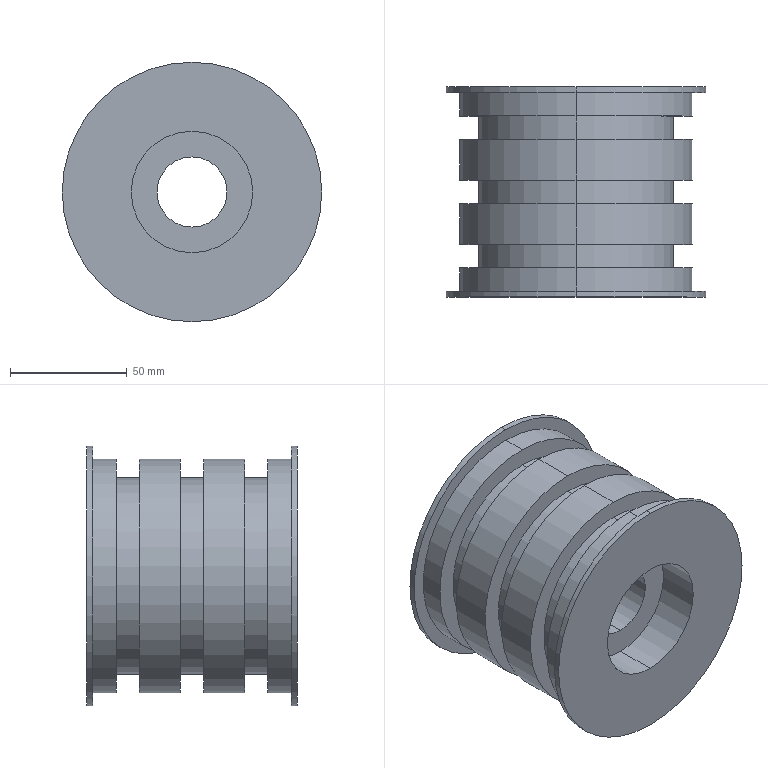Part | STEP file | 012-6-07-015 | 1 solid | 36 faces | box 111 x 90 x 111 mm | volume 531982 mm3 | cylinder 24 | plane 12 | commonest cylinder face diameters 100 x8 84 x6 52 x4 111 x4 30 x2